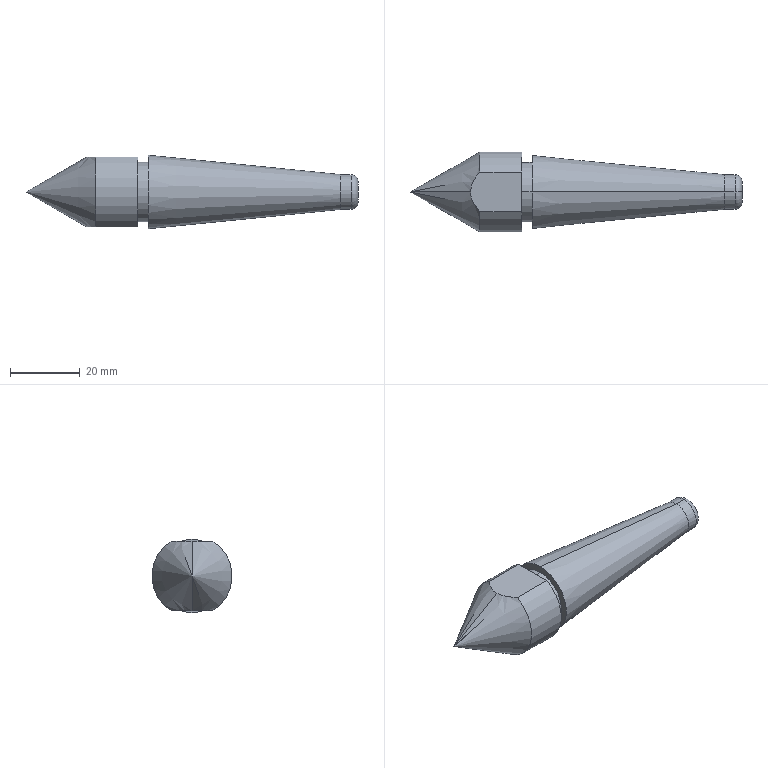Part | SolidWorks | features Fillet 1, ICE 1, Revolution 1 | 1 solid | 17 faces | box 94.92 x 23 x 21 mm | volume 19307 mm3 | cylinder 6 | plane 5 | cone 4 | torus 2 | commonest cylinder face diameters 10 x2 17 x2 23 x2
STEP:
#1=CARTESIAN_POINT('',(0.,0.,-3.));
#2=VERTEX_POINT('',#1);
#3=CARTESIAN_POINT('',(0.,0.,3.));
#4=VERTEX_POINT('',#3);
#5=CARTESIAN_POINT('',(0.,0.,0.));
#6=DIRECTION('',(1.,0.,0.));
#7=DIRECTION('',(0.,0.,1.));
#8=AXIS2_PLACEMENT_3D('',#5,#6,#7);
#9=CIRCLE('',#8,3.);
#10=EDGE_CURVE('',#2,#4,#9,.T.);
#11=ORIENTED_EDGE('',*,*,#10,.F.);
#12=CARTESIAN_POINT('',(-2.,0.,-5.));
#13=VERTEX_POINT('',#12);
#14=CARTESIAN_POINT('',(-2.,0.,-3.));
#15=DIRECTION('',(0.,1.,0.));
#16=DIRECTION('',(0.,0.,1.));
#17=AXIS2_PLACEMENT_3D('',#14,#15,#16);
#18=CIRCLE('',#17,2.);
#19=EDGE_CURVE('',#2,#13,#18,.T.);
#20=ORIENTED_EDGE('',*,*,#19,.T.);
#21=CARTESIAN_POINT('',(-2.,0.,5.));
#22=VERTEX_POINT('',#21);
#23=CARTESIAN_POINT('',(-2.,0.,0.));
#24=DIRECTION('',(-1.,0.,0.));
#25=DIRECTION('',(0.,0.,1.));
#26=AXIS2_PLACEMENT_3D('',#23,#24,#25);
#27=CIRCLE('',#26,5.);
#28=EDGE_CURVE('',#22,#13,#27,.T.);
#29=ORIENTED_EDGE('',*,*,#28,.F.);
#30=CARTESIAN_POINT('',(-2.,0.,3.));
#31=DIRECTION('',(0.,-1.,0.));
#32=DIRECTION('',(0.,0.,-1.));
#33=AXIS2_PLACEMENT_3D('',#30,#31,#32);
#34=CIRCLE('',#33,2.);
#35=EDGE_CURVE('',#4,#22,#34,.T.);
#36=ORIENTED_EDGE('',*,*,#35,.F.);
#37=EDGE_LOOP('',(#11,#20,#29,#36));
#38=FACE_OUTER_BOUND('',#37,.T.);
#39=CARTESIAN_POINT('',(-2.,0.,0.));
#40=DIRECTION('',(-1.,0.,0.));
#41=DIRECTION('',(0.,0.,1.));
#42=AXIS2_PLACEMENT_3D('',#39,#40,#41);
#43=TOROIDAL_SURFACE('',#42,3.,2.);
#44=ADVANCED_FACE('',(#38),#43,.T.);
#45=CARTESIAN_POINT('',(-94.92,0.,0.));
#46=VERTEX_POINT('',#45);
#47=CARTESIAN_POINT('',(-77.598,0.,-10.));
#48=VERTEX_POINT('',#47);
#49=CARTESIAN_POINT('',(-75.,0.,-11.5));
#50=DIRECTION('',(0.866,0.,-0.5));
#51=VECTOR('',#50,1000.);
#52=LINE('',#49,#51);
#53=EDGE_CURVE('',#46,#48,#52,.T.);
#54=ORIENTED_EDGE('',*,*,#53,.F.);
#55=CARTESIAN_POINT('',(-77.598,0.,10.));
#56=VERTEX_POINT('',#55);
#57=CARTESIAN_POINT('',(-75.,0.,11.5));
#58=DIRECTION('',(0.866,0.,0.5));
#59=VECTOR('',#58,1000.);
#60=LINE('',#57,#59);
#61=EDGE_CURVE('',#46,#56,#60,.T.);
#62=ORIENTED_EDGE('',*,*,#61,.T.);
#63=CARTESIAN_POINT('',(-75.,5.679,10.));
#64=VERTEX_POINT('',#63);
#65=CARTESIAN_POINT('',(-77.598,0.,10.));
#66=CARTESIAN_POINT('',(-77.598,0.5354,10.));
#67=CARTESIAN_POINT('',(-77.524,1.06,10.));
#68=CARTESIAN_POINT('',(-77.315,1.833,10.));
#69=CARTESIAN_POINT('',(-77.229,2.089,10.));
#70=CARTESIAN_POINT('',(-77.034,2.585,10.));
#71=CARTESIAN_POINT('',(-76.924,2.826,10.));
#72=CARTESIAN_POINT('',(-76.565,3.535,10.));
#73=CARTESIAN_POINT('',(-76.286,3.986,10.));
#74=CARTESIAN_POINT('',(-75.673,4.861,10.));
#75=CARTESIAN_POINT('',(-75.343,5.278,10.));
#76=CARTESIAN_POINT('',(-75.,5.679,10.));
#77=B_SPLINE_CURVE_WITH_KNOTS('',3,(#65,#66,#67,#68,#69,#70,#71,#72,#73,#74,#75,#76),.UNSPECIFIED.,.F.,.F.,(4,2,2,2,2,4),(0.03489,0.03646,0.03725,0.03803,0.0396,0.04117),.UNSPECIFIED.);
#78=EDGE_CURVE('',#56,#64,#77,.T.);
#79=ORIENTED_EDGE('',*,*,#78,.T.);
#80=CARTESIAN_POINT('',(-75.,5.679,-10.));
#81=VERTEX_POINT('',#80);
#82=CARTESIAN_POINT('',(-75.,0.,0.));
#83=DIRECTION('',(-1.,0.,0.));
#84=DIRECTION('',(0.,0.,1.));
#85=AXIS2_PLACEMENT_3D('',#82,#83,#84);
#86=CIRCLE('',#85,11.5);
#87=EDGE_CURVE('',#64,#81,#86,.T.);
#88=ORIENTED_EDGE('',*,*,#87,.T.);
#89=CARTESIAN_POINT('',(-75.,5.679,-10.));
#90=CARTESIAN_POINT('',(-75.342,5.28,-10.));
#91=CARTESIAN_POINT('',(-75.671,4.863,-10.));
#92=CARTESIAN_POINT('',(-76.284,3.989,-10.));
#93=CARTESIAN_POINT('',(-76.563,3.537,-10.));
#94=CARTESIAN_POINT('',(-77.044,2.59,-10.));
#95=CARTESIAN_POINT('',(-77.246,2.089,-10.));
#96=CARTESIAN_POINT('',(-77.453,1.321,-10.));
#97=CARTESIAN_POINT('',(-77.507,1.062,-10.));
#98=CARTESIAN_POINT('',(-77.579,0.5359,-10.));
#99=CARTESIAN_POINT('',(-77.598,0.2672,-10.));
#100=CARTESIAN_POINT('',(-77.598,0.,-10.));
#101=B_SPLINE_CURVE_WITH_KNOTS('',3,(#89,#90,#91,#92,#93,#94,#95,#96,#97,#98,#99,#100),.UNSPECIFIED.,.F.,.F.,(4,2,2,2,2,4),(0.02862,0.03019,0.03176,0.03332,0.03411,0.03489),.UNSPECIFIED.);
#102=EDGE_CURVE('',#81,#48,#101,.T.);
#103=ORIENTED_EDGE('',*,*,#102,.T.);
#104=EDGE_LOOP('',(#54,#62,#79,#88,#103));
#105=FACE_OUTER_BOUND('',#104,.T.);
#106=CARTESIAN_POINT('',(-75.,0.,0.));
#107=DIRECTION('',(1.,0.,0.));
#108=DIRECTION('',(0.,0.,-1.));
#109=AXIS2_PLACEMENT_3D('',#106,#107,#108);
#110=CONICAL_SURFACE('',#109,11.5,0.5236);
#111=ADVANCED_FACE('',(#105),#110,.T.);
#112=CARTESIAN_POINT('',(-60.,0.,8.5));
#113=VERTEX_POINT('',#112);
#114=CARTESIAN_POINT('',(-60.,0.,-8.5));
#115=VERTEX_POINT('',#114);
#116=CARTESIAN_POINT('',(-60.,0.,0.));
#117=DIRECTION('',(-1.,0.,0.));
#118=DIRECTION('',(0.,0.,1.));
#119=AXIS2_PLACEMENT_3D('',#116,#117,#118);
#120=CIRCLE('',#119,8.5);
#121=EDGE_CURVE('',#113,#115,#120,.T.);
#122=ORIENTED_EDGE('',*,*,#121,.T.);
#123=CARTESIAN_POINT('',(-63.,0.,-8.5));
#124=VERTEX_POINT('',#123);
#125=CARTESIAN_POINT('',(-94.92,0.,-8.5));
#126=DIRECTION('',(-1.,0.,0.));
#127=VECTOR('',#126,1000.);
#128=LINE('',#125,#127);
#129=EDGE_CURVE('',#115,#124,#128,.T.);
#130=ORIENTED_EDGE('',*,*,#129,.T.);
#131=CARTESIAN_POINT('',(-63.,0.,8.5));
#132=VERTEX_POINT('',#131);
#133=CARTESIAN_POINT('',(-63.,0.,0.));
#134=DIRECTION('',(-1.,0.,0.));
#135=DIRECTION('',(0.,0.,1.));
#136=AXIS2_PLACEMENT_3D('',#133,#134,#135);
#137=CIRCLE('',#136,8.5);
#138=EDGE_CURVE('',#132,#124,#137,.T.);
#139=ORIENTED_EDGE('',*,*,#138,.F.);
#140=CARTESIAN_POINT('',(-94.92,0.,8.5));
#141=DIRECTION('',(-1.,0.,0.));
#142=VECTOR('',#141,1000.);
#143=LINE('',#140,#142);
#144=EDGE_CURVE('',#113,#132,#143,.T.);
#145=ORIENTED_EDGE('',*,*,#144,.F.);
#146=EDGE_LOOP('',(#122,#130,#139,#145));
#147=FACE_OUTER_BOUND('',#146,.T.);
#148=CARTESIAN_POINT('',(-94.92,0.,0.));
#149=DIRECTION('',(-1.,0.,0.));
#150=DIRECTION('',(0.,0.,1.));
#151=AXIS2_PLACEMENT_3D('',#148,#149,#150);
#152=CYLINDRICAL_SURFACE('',#151,8.5);
#153=ADVANCED_FACE('',(#147),#152,.T.);
#154=CARTESIAN_POINT('',(-5.,0.,5.));
#155=VERTEX_POINT('',#154);
#156=CARTESIAN_POINT('',(-5.,0.,-5.));
#157=VERTEX_POINT('',#156);
#158=CARTESIAN_POINT('',(-5.,0.,0.));
#159=DIRECTION('',(-1.,0.,0.));
#160=DIRECTION('',(0.,0.,1.));
#161=AXIS2_PLACEMENT_3D('',#158,#159,#160);
#162=CIRCLE('',#161,5.);
#163=EDGE_CURVE('',#155,#157,#162,.T.);
#164=ORIENTED_EDGE('',*,*,#163,.T.);
#165=CARTESIAN_POINT('',(-60.,0.,-10.5));
#166=VERTEX_POINT('',#165);
#167=CARTESIAN_POINT('',(-5.,0.,-5.));
#168=DIRECTION('',(-0.995,0.,-0.0995));
#169=VECTOR('',#168,1000.);
#170=LINE('',#167,#169);
#171=EDGE_CURVE('',#157,#166,#170,.T.);
#172=ORIENTED_EDGE('',*,*,#171,.T.);
#173=CARTESIAN_POINT('',(-60.,0.,10.5));
#174=VERTEX_POINT('',#173);
#175=CARTESIAN_POINT('',(-60.,0.,0.));
#176=DIRECTION('',(-1.,0.,0.));
#177=DIRECTION('',(0.,0.,1.));
#178=AXIS2_PLACEMENT_3D('',#175,#176,#177);
#179=CIRCLE('',#178,10.5);
#180=EDGE_CURVE('',#174,#166,#179,.T.);
#181=ORIENTED_EDGE('',*,*,#180,.F.);
#182=CARTESIAN_POINT('',(-5.,0.,5.));
#183=DIRECTION('',(-0.995,0.,0.0995));
#184=VECTOR('',#183,1000.);
#185=LINE('',#182,#184);
#186=EDGE_CURVE('',#155,#174,#185,.T.);
#187=ORIENTED_EDGE('',*,*,#186,.F.);
#188=EDGE_LOOP('',(#164,#172,#181,#187));
#189=FACE_OUTER_BOUND('',#188,.T.);
#190=CARTESIAN_POINT('',(-5.,0.,0.));
#191=DIRECTION('',(-1.,0.,0.));
#192=DIRECTION('',(0.,0.,1.));
#193=AXIS2_PLACEMENT_3D('',#190,#191,#192);
#194=CONICAL_SURFACE('',#193,5.,0.09967);
#195=ADVANCED_FACE('',(#189),#194,.T.);
#196=ORIENTED_EDGE('',*,*,#28,.T.);
#197=CARTESIAN_POINT('',(-94.92,0.,-5.));
#198=DIRECTION('',(-1.,0.,0.));
#199=VECTOR('',#198,1000.);
#200=LINE('',#197,#199);
#201=EDGE_CURVE('',#13,#157,#200,.T.);
#202=ORIENTED_EDGE('',*,*,#201,.T.);
#203=ORIENTED_EDGE('',*,*,#163,.F.);
#204=CARTESIAN_POINT('',(-94.92,0.,5.));
#205=DIRECTION('',(-1.,0.,0.));
#206=VECTOR('',#205,1000.);
#207=LINE('',#204,#206);
#208=EDGE_CURVE('',#22,#155,#207,.T.);
#209=ORIENTED_EDGE('',*,*,#208,.F.);
#210=EDGE_LOOP('',(#196,#202,#203,#209));
#211=FACE_OUTER_BOUND('',#210,.T.);
#212=CARTESIAN_POINT('',(-94.92,0.,0.));
#213=DIRECTION('',(-1.,0.,0.));
#214=DIRECTION('',(0.,0.,1.));
#215=AXIS2_PLACEMENT_3D('',#212,#213,#214);
#216=CYLINDRICAL_SURFACE('',#215,5.);
#217=ADVANCED_FACE('',(#211),#216,.T.);
#218=CARTESIAN_POINT('',(-63.,5.679,10.));
#219=VERTEX_POINT('',#218);
#220=CARTESIAN_POINT('',(-63.,5.679,-10.));
#221=VERTEX_POINT('',#220);
#222=CARTESIAN_POINT('',(-63.,0.,0.));
#223=DIRECTION('',(-1.,0.,0.));
#224=DIRECTION('',(0.,0.,1.));
#225=AXIS2_PLACEMENT_3D('',#222,#223,#224);
#226=CIRCLE('',#225,11.5);
#227=EDGE_CURVE('',#219,#221,#226,.T.);
#228=ORIENTED_EDGE('',*,*,#227,.T.);
#229=CARTESIAN_POINT('',(-94.92,5.679,-10.));
#230=DIRECTION('',(1.,0.,0.));
#231=VECTOR('',#230,1000.);
#232=LINE('',#229,#231);
#233=EDGE_CURVE('',#81,#221,#232,.T.);
#234=ORIENTED_EDGE('',*,*,#233,.F.);
#235=ORIENTED_EDGE('',*,*,#87,.F.);
#236=CARTESIAN_POINT('',(-94.92,5.679,10.));
#237=DIRECTION('',(1.,0.,0.));
#238=VECTOR('',#237,1000.);
#239=LINE('',#236,#238);
#240=EDGE_CURVE('',#64,#219,#239,.T.);
#241=ORIENTED_EDGE('',*,*,#240,.T.);
#242=EDGE_LOOP('',(#228,#234,#235,#241));
#243=FACE_OUTER_BOUND('',#242,.T.);
#244=CARTESIAN_POINT('',(-94.92,0.,0.));
#245=DIRECTION('',(-1.,0.,0.));
#246=DIRECTION('',(0.,0.,1.));
#247=AXIS2_PLACEMENT_3D('',#244,#245,#246);
#248=CYLINDRICAL_SURFACE('',#247,11.5);
#249=ADVANCED_FACE('',(#243),#248,.T.);
#250=CARTESIAN_POINT('',(0.,0.,0.));
#251=DIRECTION('',(1.,0.,0.));
#252=DIRECTION('',(0.,0.,1.));
#253=AXIS2_PLACEMENT_3D('',#250,#251,#252);
#254=CIRCLE('',#253,3.);
#255=EDGE_CURVE('',#4,#2,#254,.T.);
#256=ORIENTED_EDGE('',*,*,#255,.T.);
#257=ORIENTED_EDGE('',*,*,#10,.T.);
#258=EDGE_LOOP('',(#256,#257));
#259=FACE_OUTER_BOUND('',#258,.T.);
#260=CARTESIAN_POINT('',(0.,0.,0.));
#261=DIRECTION('',(-1.,0.,0.));
#262=DIRECTION('',(0.,0.,1.));
#263=AXIS2_PLACEMENT_3D('',#260,#261,#262);
#264=PLANE('',#263);
#265=ADVANCED_FACE('',(#259),#264,.F.);
#266=ORIENTED_EDGE('',*,*,#201,.F.);
#267=CARTESIAN_POINT('',(-2.,0.,0.));
#268=DIRECTION('',(-1.,0.,0.));
#269=DIRECTION('',(0.,0.,1.));
#270=AXIS2_PLACEMENT_3D('',#267,#268,#269);
#271=CIRCLE('',#270,5.);
#272=EDGE_CURVE('',#13,#22,#271,.T.);
#273=ORIENTED_EDGE('',*,*,#272,.T.);
#274=ORIENTED_EDGE('',*,*,#208,.T.);
#275=CARTESIAN_POINT('',(-5.,0.,0.));
#276=DIRECTION('',(-1.,0.,0.));
#277=DIRECTION('',(0.,0.,1.));
#278=AXIS2_PLACEMENT_3D('',#275,#276,#277);
#279=CIRCLE('',#278,5.);
#280=EDGE_CURVE('',#157,#155,#279,.T.);
#281=ORIENTED_EDGE('',*,*,#280,.F.);
#282=EDGE_LOOP('',(#266,#273,#274,#281));
#283=FACE_OUTER_BOUND('',#282,.T.);
#284=CARTESIAN_POINT('',(-94.92,0.,0.));
#285=DIRECTION('',(-1.,0.,0.));
#286=DIRECTION('',(0.,0.,1.));
#287=AXIS2_PLACEMENT_3D('',#284,#285,#286);
#288=CYLINDRICAL_SURFACE('',#287,5.);
#289=ADVANCED_FACE('',(#283),#288,.T.);
#290=ORIENTED_EDGE('',*,*,#171,.F.);
#291=ORIENTED_EDGE('',*,*,#280,.T.);
#292=ORIENTED_EDGE('',*,*,#186,.T.);
#293=CARTESIAN_POINT('',(-60.,0.,0.));
#294=DIRECTION('',(-1.,0.,0.));
#295=DIRECTION('',(0.,0.,1.));
#296=AXIS2_PLACEMENT_3D('',#293,#294,#295);
#297=CIRCLE('',#296,10.5);
#298=EDGE_CURVE('',#166,#174,#297,.T.);
#299=ORIENTED_EDGE('',*,*,#298,.F.);
#300=EDGE_LOOP('',(#290,#291,#292,#299));
#301=FACE_OUTER_BOUND('',#300,.T.);
#302=CARTESIAN_POINT('',(-5.,0.,0.));
#303=DIRECTION('',(-1.,0.,0.));
#304=DIRECTION('',(0.,0.,1.));
#305=AXIS2_PLACEMENT_3D('',#302,#303,#304);
#306=CONICAL_SURFACE('',#305,5.,0.09967);
#307=ADVANCED_FACE('',(#301),#306,.T.);
#308=ORIENTED_EDGE('',*,*,#121,.F.);
#309=CARTESIAN_POINT('',(-60.,0.,0.));
#310=DIRECTION('',(-1.,0.,0.));
#311=DIRECTION('',(0.,0.,1.));
#312=AXIS2_PLACEMENT_3D('',#309,#310,#311);
#313=CIRCLE('',#312,8.5);
#314=EDGE_CURVE('',#115,#113,#313,.T.);
#315=ORIENTED_EDGE('',*,*,#314,.F.);
#316=EDGE_LOOP('',(#308,#315));
#317=FACE_BOUND('',#316,.T.);
#318=ORIENTED_EDGE('',*,*,#180,.T.);
#319=ORIENTED_EDGE('',*,*,#298,.T.);
#320=EDGE_LOOP('',(#318,#319));
#321=FACE_OUTER_BOUND('',#320,.T.);
#322=CARTESIAN_POINT('',(-60.,10.5,0.));
#323=DIRECTION('',(1.,0.,0.));
#324=DIRECTION('',(0.,0.,-1.));
#325=AXIS2_PLACEMENT_3D('',#322,#323,#324);
#326=PLANE('',#325);
#327=ADVANCED_FACE('',(#317,#321),#326,.F.);
#328=ORIENTED_EDGE('',*,*,#129,.F.);
#329=ORIENTED_EDGE('',*,*,#314,.T.);
#330=ORIENTED_EDGE('',*,*,#144,.T.);
#331=CARTESIAN_POINT('',(-63.,0.,0.));
#332=DIRECTION('',(-1.,0.,0.));
#333=DIRECTION('',(0.,0.,1.));
#334=AXIS2_PLACEMENT_3D('',#331,#332,#333);
#335=CIRCLE('',#334,8.5);
#336=EDGE_CURVE('',#124,#132,#335,.T.);
#337=ORIENTED_EDGE('',*,*,#336,.F.);
#338=EDGE_LOOP('',(#328,#329,#330,#337));
#339=FACE_OUTER_BOUND('',#338,.T.);
#340=CARTESIAN_POINT('',(-94.92,0.,0.));
#341=DIRECTION('',(-1.,0.,0.));
#342=DIRECTION('',(0.,0.,1.));
#343=AXIS2_PLACEMENT_3D('',#340,#341,#342);
#344=CYLINDRICAL_SURFACE('',#343,8.5);
#345=ADVANCED_FACE('',(#339),#344,.T.);
#346=CARTESIAN_POINT('',(-63.,-5.679,-10.));
#347=VERTEX_POINT('',#346);
#348=CARTESIAN_POINT('',(-63.,-5.679,10.));
#349=VERTEX_POINT('',#348);
#350=CARTESIAN_POINT('',(-63.,0.,0.));
#351=DIRECTION('',(-1.,0.,0.));
#352=DIRECTION('',(0.,0.,1.));
#353=AXIS2_PLACEMENT_3D('',#350,#351,#352);
#354=CIRCLE('',#353,11.5);
#355=EDGE_CURVE('',#347,#349,#354,.T.);
#356=ORIENTED_EDGE('',*,*,#355,.F.);
#357=CARTESIAN_POINT('',(-63.,5.679,-10.));
#358=DIRECTION('',(0.,-1.,0.));
#359=VECTOR('',#358,1000.);
#360=LINE('',#357,#359);
#361=EDGE_CURVE('',#221,#347,#360,.T.);
#362=ORIENTED_EDGE('',*,*,#361,.F.);
#363=ORIENTED_EDGE('',*,*,#227,.F.);
#364=CARTESIAN_POINT('',(-63.,5.679,10.));
#365=DIRECTION('',(0.,1.,0.));
#366=VECTOR('',#365,1000.);
#367=LINE('',#364,#366);
#368=EDGE_CURVE('',#349,#219,#367,.T.);
#369=ORIENTED_EDGE('',*,*,#368,.F.);
#370=EDGE_LOOP('',(#356,#362,#363,#369));
#371=FACE_OUTER_BOUND('',#370,.T.);
#372=ORIENTED_EDGE('',*,*,#138,.T.);
#373=ORIENTED_EDGE('',*,*,#336,.T.);
#374=EDGE_LOOP('',(#372,#373));
#375=FACE_BOUND('',#374,.T.);
#376=CARTESIAN_POINT('',(-63.,8.5,0.));
#377=DIRECTION('',(-1.,0.,0.));
#378=DIRECTION('',(0.,0.,1.));
#379=AXIS2_PLACEMENT_3D('',#376,#377,#378);
#380=PLANE('',#379);
#381=ADVANCED_FACE('',(#371,#375),#380,.F.);
#382=CARTESIAN_POINT('',(-75.,-5.679,-10.));
#383=VERTEX_POINT('',#382);
#384=CARTESIAN_POINT('',(-75.,-5.679,10.));
#385=VERTEX_POINT('',#384);
#386=CARTESIAN_POINT('',(-75.,0.,0.));
#387=DIRECTION('',(-1.,0.,0.));
#388=DIRECTION('',(0.,0.,1.));
#389=AXIS2_PLACEMENT_3D('',#386,#387,#388);
#390=CIRCLE('',#389,11.5);
#391=EDGE_CURVE('',#383,#385,#390,.T.);
#392=ORIENTED_EDGE('',*,*,#391,.F.);
#393=CARTESIAN_POINT('',(-94.92,-5.679,-10.));
#394=DIRECTION('',(1.,0.,0.));
#395=VECTOR('',#394,1000.);
#396=LINE('',#393,#395);
#397=EDGE_CURVE('',#383,#347,#396,.T.);
#398=ORIENTED_EDGE('',*,*,#397,.T.);
#399=ORIENTED_EDGE('',*,*,#355,.T.);
#400=CARTESIAN_POINT('',(-94.92,-5.679,10.));
#401=DIRECTION('',(1.,0.,0.));
#402=VECTOR('',#401,1000.);
#403=LINE('',#400,#402);
#404=EDGE_CURVE('',#385,#349,#403,.T.);
#405=ORIENTED_EDGE('',*,*,#404,.F.);
#406=EDGE_LOOP('',(#392,#398,#399,#405));
#407=FACE_OUTER_BOUND('',#406,.T.);
#408=CARTESIAN_POINT('',(-94.92,0.,0.));
#409=DIRECTION('',(-1.,0.,0.));
#410=DIRECTION('',(0.,0.,1.));
#411=AXIS2_PLACEMENT_3D('',#408,#409,#410);
#412=CYLINDRICAL_SURFACE('',#411,11.5);
#413=ADVANCED_FACE('',(#407),#412,.T.);
#414=ORIENTED_EDGE('',*,*,#61,.F.);
#415=ORIENTED_EDGE('',*,*,#53,.T.);
#416=CARTESIAN_POINT('',(-77.598,0.,-10.));
#417=CARTESIAN_POINT('',(-77.598,-0.5354,-10.));
#418=CARTESIAN_POINT('',(-77.524,-1.06,-10.));
#419=CARTESIAN_POINT('',(-77.315,-1.833,-10.));
#420=CARTESIAN_POINT('',(-77.229,-2.089,-10.));
#421=CARTESIAN_POINT('',(-77.034,-2.585,-10.));
#422=CARTESIAN_POINT('',(-76.924,-2.826,-10.));
#423=CARTESIAN_POINT('',(-76.565,-3.535,-10.));
#424=CARTESIAN_POINT('',(-76.286,-3.986,-10.));
#425=CARTESIAN_POINT('',(-75.673,-4.861,-10.));
#426=CARTESIAN_POINT('',(-75.343,-5.278,-10.));
#427=CARTESIAN_POINT('',(-75.,-5.679,-10.));
#428=B_SPLINE_CURVE_WITH_KNOTS('',3,(#416,#417,#418,#419,#420,#421,#422,#423,#424,#425,#426,#427),.UNSPECIFIED.,.F.,.F.,(4,2,2,2,2,4),(0.03489,0.03646,0.03725,0.03803,0.0396,0.04117),.UNSPECIFIED.);
#429=EDGE_CURVE('',#48,#383,#428,.T.);
#430=ORIENTED_EDGE('',*,*,#429,.T.);
#431=ORIENTED_EDGE('',*,*,#391,.T.);
#432=CARTESIAN_POINT('',(-75.,-5.679,10.));
#433=CARTESIAN_POINT('',(-75.342,-5.28,10.));
#434=CARTESIAN_POINT('',(-75.671,-4.863,10.));
#435=CARTESIAN_POINT('',(-76.284,-3.989,10.));
#436=CARTESIAN_POINT('',(-76.563,-3.537,10.));
#437=CARTESIAN_POINT('',(-77.044,-2.59,10.));
#438=CARTESIAN_POINT('',(-77.246,-2.089,10.));
#439=CARTESIAN_POINT('',(-77.453,-1.321,10.));
#440=CARTESIAN_POINT('',(-77.507,-1.062,10.));
#441=CARTESIAN_POINT('',(-77.579,-0.5359,10.));
#442=CARTESIAN_POINT('',(-77.598,-0.2672,10.));
#443=CARTESIAN_POINT('',(-77.598,0.,10.));
#444=B_SPLINE_CURVE_WITH_KNOTS('',3,(#432,#433,#434,#435,#436,#437,#438,#439,#440,#441,#442,#443),.UNSPECIFIED.,.F.,.F.,(4,2,2,2,2,4),(0.02862,0.03019,0.03176,0.03332,0.03411,0.03489),.UNSPECIFIED.);
#445=EDGE_CURVE('',#385,#56,#444,.T.);
#446=ORIENTED_EDGE('',*,*,#445,.T.);
#447=EDGE_LOOP('',(#414,#415,#430,#431,#446));
#448=FACE_OUTER_BOUND('',#447,.T.);
#449=CARTESIAN_POINT('',(-75.,0.,0.));
#450=DIRECTION('',(1.,0.,0.));
#451=DIRECTION('',(0.,0.,-1.));
#452=AXIS2_PLACEMENT_3D('',#449,#450,#451);
#453=CONICAL_SURFACE('',#452,11.5,0.5236);
#454=ADVANCED_FACE('',(#448),#453,.T.);
#455=ORIENTED_EDGE('',*,*,#19,.F.);
#456=ORIENTED_EDGE('',*,*,#255,.F.);
#457=ORIENTED_EDGE('',*,*,#35,.T.);
#458=ORIENTED_EDGE('',*,*,#272,.F.);
#459=EDGE_LOOP('',(#455,#456,#457,#458));
#460=FACE_OUTER_BOUND('',#459,.T.);
#461=CARTESIAN_POINT('',(-2.,0.,0.));
#462=DIRECTION('',(-1.,0.,0.));
#463=DIRECTION('',(0.,0.,1.));
#464=AXIS2_PLACEMENT_3D('',#461,#462,#463);
#465=TOROIDAL_SURFACE('',#464,3.,2.);
#466=ADVANCED_FACE('',(#460),#465,.T.);
#467=ORIENTED_EDGE('',*,*,#404,.T.);
#468=ORIENTED_EDGE('',*,*,#368,.T.);
#469=ORIENTED_EDGE('',*,*,#240,.F.);
#470=ORIENTED_EDGE('',*,*,#78,.F.);
#471=ORIENTED_EDGE('',*,*,#445,.F.);
#472=EDGE_LOOP('',(#467,#468,#469,#470,#471));
#473=FACE_OUTER_BOUND('',#472,.T.);
#474=CARTESIAN_POINT('',(-94.92,5.679,10.));
#475=DIRECTION('',(0.,0.,-1.));
#476=DIRECTION('',(0.,1.,0.));
#477=AXIS2_PLACEMENT_3D('',#474,#475,#476);
#478=PLANE('',#477);
#479=ADVANCED_FACE('',(#473),#478,.F.);
#480=ORIENTED_EDGE('',*,*,#233,.T.);
#481=ORIENTED_EDGE('',*,*,#361,.T.);
#482=ORIENTED_EDGE('',*,*,#397,.F.);
#483=ORIENTED_EDGE('',*,*,#429,.F.);
#484=ORIENTED_EDGE('',*,*,#102,.F.);
#485=EDGE_LOOP('',(#480,#481,#482,#483,#484));
#486=FACE_OUTER_BOUND('',#485,.T.);
#487=CARTESIAN_POINT('',(-94.92,5.679,-10.));
#488=DIRECTION('',(0.,0.,1.));
#489=DIRECTION('',(1.,0.,0.));
#490=AXIS2_PLACEMENT_3D('',#487,#488,#489);
#491=PLANE('',#490);
#492=ADVANCED_FACE('',(#486),#491,.F.);
#493=CLOSED_SHELL('',(#44,#111,#153,#195,#217,#249,#265,#289,#307,#327,#345,#381,#413,#454,#466,#479,#492));
#494=MANIFOLD_SOLID_BREP('',#493);
#495=CARTESIAN_POINT('',(0.,0.,0.));
#496=DIRECTION('',(0.,0.,1.));
#497=DIRECTION('',(1.,0.,0.));
#498=AXIS2_PLACEMENT_3D('',#495,#496,#497);
#499=(LENGTH_UNIT()NAMED_UNIT(*)SI_UNIT(.MILLI.,.METRE.));
#500=UNCERTAINTY_MEASURE_WITH_UNIT(LENGTH_MEASURE(0.00001),#499,'','');
#501=(NAMED_UNIT(*)PLANE_ANGLE_UNIT()SI_UNIT($,.RADIAN.));
#502=(NAMED_UNIT(*)SI_UNIT($,.STERADIAN.)SOLID_ANGLE_UNIT());
#503=(GEOMETRIC_REPRESENTATION_CONTEXT(3)GLOBAL_UNCERTAINTY_ASSIGNED_CONTEXT((#500))GLOBAL_UNIT_ASSIGNED_CONTEXT((#499,#501,#502))REPRESENTATION_CONTEXT('',''));
#504=ADVANCED_BREP_SHAPE_REPRESENTATION('',(#494,#498),#503);